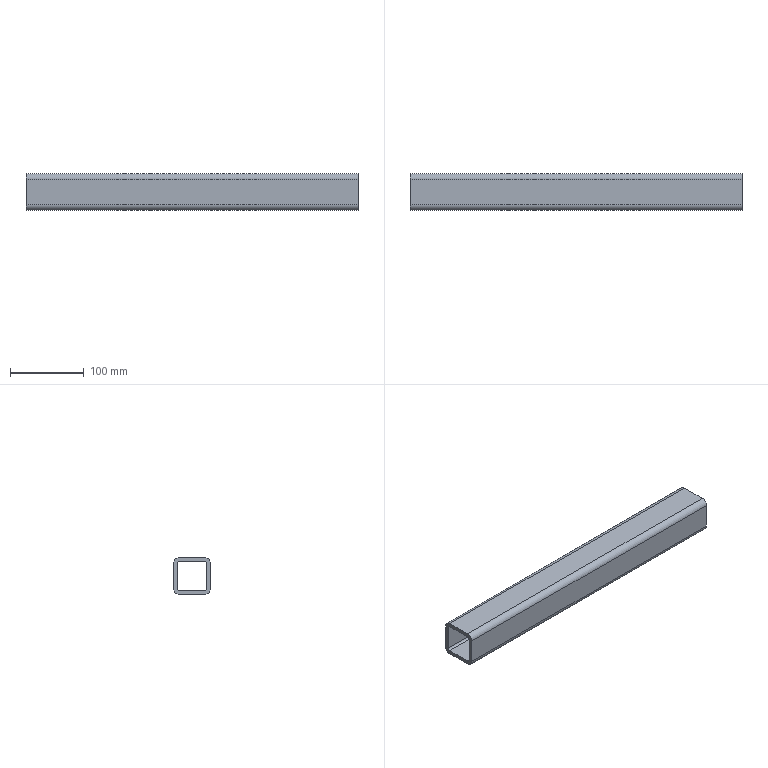Part | SolidWorks | features WeldMemberFeat 1, WeldmentFeature 1 | 1 solid | 18 faces | box 450 x 50 x 50 mm | volume 383754 mm3 | plane 10 | cylinder 8 | commonest cylinder face diameters 6 x4 16 x4
STEP:
#1=CARTESIAN_POINT('',(-88.434,25.,17.));
#2=VERTEX_POINT('',#1);
#3=CARTESIAN_POINT('',(-88.434,17.,25.));
#4=VERTEX_POINT('',#3);
#5=CARTESIAN_POINT('',(-88.434,17.,17.));
#6=DIRECTION('',(1.,0.,0.));
#7=DIRECTION('',(0.,0.,-1.));
#8=AXIS2_PLACEMENT_3D('',#5,#6,#7);
#9=CIRCLE('',#8,8.);
#10=EDGE_CURVE('',#2,#4,#9,.T.);
#11=ORIENTED_EDGE('',*,*,#10,.T.);
#12=CARTESIAN_POINT('',(361.566,17.,25.));
#13=VERTEX_POINT('',#12);
#14=CARTESIAN_POINT('',(361.566,17.,25.));
#15=DIRECTION('',(-1.,0.,0.));
#16=VECTOR('',#15,1000.);
#17=LINE('',#14,#16);
#18=EDGE_CURVE('',#13,#4,#17,.T.);
#19=ORIENTED_EDGE('',*,*,#18,.F.);
#20=CARTESIAN_POINT('',(361.566,25.,17.));
#21=VERTEX_POINT('',#20);
#22=CARTESIAN_POINT('',(361.566,17.,17.));
#23=DIRECTION('',(1.,0.,0.));
#24=DIRECTION('',(0.,0.,-1.));
#25=AXIS2_PLACEMENT_3D('',#22,#23,#24);
#26=CIRCLE('',#25,8.);
#27=EDGE_CURVE('',#21,#13,#26,.T.);
#28=ORIENTED_EDGE('',*,*,#27,.F.);
#29=CARTESIAN_POINT('',(361.566,25.,17.));
#30=DIRECTION('',(-1.,0.,0.));
#31=VECTOR('',#30,1000.);
#32=LINE('',#29,#31);
#33=EDGE_CURVE('',#21,#2,#32,.T.);
#34=ORIENTED_EDGE('',*,*,#33,.T.);
#35=EDGE_LOOP('',(#11,#19,#28,#34));
#36=FACE_OUTER_BOUND('',#35,.T.);
#37=CARTESIAN_POINT('',(361.566,17.,17.));
#38=DIRECTION('',(-1.,0.,0.));
#39=DIRECTION('',(0.,0.,1.));
#40=AXIS2_PLACEMENT_3D('',#37,#38,#39);
#41=CYLINDRICAL_SURFACE('',#40,8.);
#42=ADVANCED_FACE('',(#36),#41,.T.);
#43=CARTESIAN_POINT('',(-88.434,-17.,25.));
#44=VERTEX_POINT('',#43);
#45=CARTESIAN_POINT('',(-88.434,17.,25.));
#46=DIRECTION('',(0.,-1.,0.));
#47=VECTOR('',#46,1000.);
#48=LINE('',#45,#47);
#49=EDGE_CURVE('',#4,#44,#48,.T.);
#50=ORIENTED_EDGE('',*,*,#49,.T.);
#51=CARTESIAN_POINT('',(361.566,-17.,25.));
#52=VERTEX_POINT('',#51);
#53=CARTESIAN_POINT('',(361.566,-17.,25.));
#54=DIRECTION('',(-1.,0.,0.));
#55=VECTOR('',#54,1000.);
#56=LINE('',#53,#55);
#57=EDGE_CURVE('',#52,#44,#56,.T.);
#58=ORIENTED_EDGE('',*,*,#57,.F.);
#59=CARTESIAN_POINT('',(361.566,17.,25.));
#60=DIRECTION('',(0.,-1.,0.));
#61=VECTOR('',#60,1000.);
#62=LINE('',#59,#61);
#63=EDGE_CURVE('',#13,#52,#62,.T.);
#64=ORIENTED_EDGE('',*,*,#63,.F.);
#65=ORIENTED_EDGE('',*,*,#18,.T.);
#66=EDGE_LOOP('',(#50,#58,#64,#65));
#67=FACE_OUTER_BOUND('',#66,.T.);
#68=CARTESIAN_POINT('',(361.566,17.,25.));
#69=DIRECTION('',(0.,0.,-1.));
#70=DIRECTION('',(-1.,0.,0.));
#71=AXIS2_PLACEMENT_3D('',#68,#69,#70);
#72=PLANE('',#71);
#73=ADVANCED_FACE('',(#67),#72,.F.);
#74=CARTESIAN_POINT('',(-88.434,-25.,17.));
#75=VERTEX_POINT('',#74);
#76=CARTESIAN_POINT('',(-88.434,-17.,17.));
#77=DIRECTION('',(1.,0.,0.));
#78=DIRECTION('',(0.,0.,-1.));
#79=AXIS2_PLACEMENT_3D('',#76,#77,#78);
#80=CIRCLE('',#79,8.);
#81=EDGE_CURVE('',#44,#75,#80,.T.);
#82=ORIENTED_EDGE('',*,*,#81,.T.);
#83=CARTESIAN_POINT('',(361.566,-25.,17.));
#84=VERTEX_POINT('',#83);
#85=CARTESIAN_POINT('',(361.566,-25.,17.));
#86=DIRECTION('',(-1.,0.,0.));
#87=VECTOR('',#86,1000.);
#88=LINE('',#85,#87);
#89=EDGE_CURVE('',#84,#75,#88,.T.);
#90=ORIENTED_EDGE('',*,*,#89,.F.);
#91=CARTESIAN_POINT('',(361.566,-17.,17.));
#92=DIRECTION('',(1.,0.,0.));
#93=DIRECTION('',(0.,0.,-1.));
#94=AXIS2_PLACEMENT_3D('',#91,#92,#93);
#95=CIRCLE('',#94,8.);
#96=EDGE_CURVE('',#52,#84,#95,.T.);
#97=ORIENTED_EDGE('',*,*,#96,.F.);
#98=ORIENTED_EDGE('',*,*,#57,.T.);
#99=EDGE_LOOP('',(#82,#90,#97,#98));
#100=FACE_OUTER_BOUND('',#99,.T.);
#101=CARTESIAN_POINT('',(361.566,-17.,17.));
#102=DIRECTION('',(-1.,0.,0.));
#103=DIRECTION('',(0.,0.,1.));
#104=AXIS2_PLACEMENT_3D('',#101,#102,#103);
#105=CYLINDRICAL_SURFACE('',#104,8.);
#106=ADVANCED_FACE('',(#100),#105,.T.);
#107=CARTESIAN_POINT('',(-88.434,-25.,-17.));
#108=VERTEX_POINT('',#107);
#109=CARTESIAN_POINT('',(-88.434,-25.,-17.));
#110=DIRECTION('',(0.,0.,-1.));
#111=VECTOR('',#110,1000.);
#112=LINE('',#109,#111);
#113=EDGE_CURVE('',#75,#108,#112,.T.);
#114=ORIENTED_EDGE('',*,*,#113,.T.);
#115=CARTESIAN_POINT('',(361.566,-25.,-17.));
#116=VERTEX_POINT('',#115);
#117=CARTESIAN_POINT('',(361.566,-25.,-17.));
#118=DIRECTION('',(-1.,0.,0.));
#119=VECTOR('',#118,1000.);
#120=LINE('',#117,#119);
#121=EDGE_CURVE('',#116,#108,#120,.T.);
#122=ORIENTED_EDGE('',*,*,#121,.F.);
#123=CARTESIAN_POINT('',(361.566,-25.,-17.));
#124=DIRECTION('',(0.,0.,-1.));
#125=VECTOR('',#124,1000.);
#126=LINE('',#123,#125);
#127=EDGE_CURVE('',#84,#116,#126,.T.);
#128=ORIENTED_EDGE('',*,*,#127,.F.);
#129=ORIENTED_EDGE('',*,*,#89,.T.);
#130=EDGE_LOOP('',(#114,#122,#128,#129));
#131=FACE_OUTER_BOUND('',#130,.T.);
#132=CARTESIAN_POINT('',(361.566,-25.,-17.));
#133=DIRECTION('',(0.,1.,0.));
#134=DIRECTION('',(0.,0.,1.));
#135=AXIS2_PLACEMENT_3D('',#132,#133,#134);
#136=PLANE('',#135);
#137=ADVANCED_FACE('',(#131),#136,.F.);
#138=CARTESIAN_POINT('',(-88.434,-17.,-25.));
#139=VERTEX_POINT('',#138);
#140=CARTESIAN_POINT('',(-88.434,-17.,-17.));
#141=DIRECTION('',(1.,0.,0.));
#142=DIRECTION('',(0.,0.,-1.));
#143=AXIS2_PLACEMENT_3D('',#140,#141,#142);
#144=CIRCLE('',#143,8.);
#145=EDGE_CURVE('',#108,#139,#144,.T.);
#146=ORIENTED_EDGE('',*,*,#145,.T.);
#147=CARTESIAN_POINT('',(361.566,-17.,-25.));
#148=VERTEX_POINT('',#147);
#149=CARTESIAN_POINT('',(361.566,-17.,-25.));
#150=DIRECTION('',(-1.,0.,0.));
#151=VECTOR('',#150,1000.);
#152=LINE('',#149,#151);
#153=EDGE_CURVE('',#148,#139,#152,.T.);
#154=ORIENTED_EDGE('',*,*,#153,.F.);
#155=CARTESIAN_POINT('',(361.566,-17.,-17.));
#156=DIRECTION('',(1.,0.,0.));
#157=DIRECTION('',(0.,0.,-1.));
#158=AXIS2_PLACEMENT_3D('',#155,#156,#157);
#159=CIRCLE('',#158,8.);
#160=EDGE_CURVE('',#116,#148,#159,.T.);
#161=ORIENTED_EDGE('',*,*,#160,.F.);
#162=ORIENTED_EDGE('',*,*,#121,.T.);
#163=EDGE_LOOP('',(#146,#154,#161,#162));
#164=FACE_OUTER_BOUND('',#163,.T.);
#165=CARTESIAN_POINT('',(361.566,-17.,-17.));
#166=DIRECTION('',(-1.,0.,0.));
#167=DIRECTION('',(0.,0.,1.));
#168=AXIS2_PLACEMENT_3D('',#165,#166,#167);
#169=CYLINDRICAL_SURFACE('',#168,8.);
#170=ADVANCED_FACE('',(#164),#169,.T.);
#171=CARTESIAN_POINT('',(-88.434,17.,-25.));
#172=VERTEX_POINT('',#171);
#173=CARTESIAN_POINT('',(-88.434,-17.,-25.));
#174=DIRECTION('',(0.,1.,0.));
#175=VECTOR('',#174,1000.);
#176=LINE('',#173,#175);
#177=EDGE_CURVE('',#139,#172,#176,.T.);
#178=ORIENTED_EDGE('',*,*,#177,.T.);
#179=CARTESIAN_POINT('',(361.566,17.,-25.));
#180=VERTEX_POINT('',#179);
#181=CARTESIAN_POINT('',(361.566,17.,-25.));
#182=DIRECTION('',(-1.,0.,0.));
#183=VECTOR('',#182,1000.);
#184=LINE('',#181,#183);
#185=EDGE_CURVE('',#180,#172,#184,.T.);
#186=ORIENTED_EDGE('',*,*,#185,.F.);
#187=CARTESIAN_POINT('',(361.566,-17.,-25.));
#188=DIRECTION('',(0.,1.,0.));
#189=VECTOR('',#188,1000.);
#190=LINE('',#187,#189);
#191=EDGE_CURVE('',#148,#180,#190,.T.);
#192=ORIENTED_EDGE('',*,*,#191,.F.);
#193=ORIENTED_EDGE('',*,*,#153,.T.);
#194=EDGE_LOOP('',(#178,#186,#192,#193));
#195=FACE_OUTER_BOUND('',#194,.T.);
#196=CARTESIAN_POINT('',(361.566,-17.,-25.));
#197=DIRECTION('',(0.,0.,1.));
#198=DIRECTION('',(1.,0.,0.));
#199=AXIS2_PLACEMENT_3D('',#196,#197,#198);
#200=PLANE('',#199);
#201=ADVANCED_FACE('',(#195),#200,.F.);
#202=CARTESIAN_POINT('',(-88.434,25.,-17.));
#203=VERTEX_POINT('',#202);
#204=CARTESIAN_POINT('',(-88.434,17.,-17.));
#205=DIRECTION('',(1.,0.,0.));
#206=DIRECTION('',(0.,0.,-1.));
#207=AXIS2_PLACEMENT_3D('',#204,#205,#206);
#208=CIRCLE('',#207,8.);
#209=EDGE_CURVE('',#172,#203,#208,.T.);
#210=ORIENTED_EDGE('',*,*,#209,.T.);
#211=CARTESIAN_POINT('',(361.566,25.,-17.));
#212=VERTEX_POINT('',#211);
#213=CARTESIAN_POINT('',(361.566,25.,-17.));
#214=DIRECTION('',(-1.,0.,0.));
#215=VECTOR('',#214,1000.);
#216=LINE('',#213,#215);
#217=EDGE_CURVE('',#212,#203,#216,.T.);
#218=ORIENTED_EDGE('',*,*,#217,.F.);
#219=CARTESIAN_POINT('',(361.566,17.,-17.));
#220=DIRECTION('',(1.,0.,0.));
#221=DIRECTION('',(0.,0.,-1.));
#222=AXIS2_PLACEMENT_3D('',#219,#220,#221);
#223=CIRCLE('',#222,8.);
#224=EDGE_CURVE('',#180,#212,#223,.T.);
#225=ORIENTED_EDGE('',*,*,#224,.F.);
#226=ORIENTED_EDGE('',*,*,#185,.T.);
#227=EDGE_LOOP('',(#210,#218,#225,#226));
#228=FACE_OUTER_BOUND('',#227,.T.);
#229=CARTESIAN_POINT('',(361.566,17.,-17.));
#230=DIRECTION('',(-1.,0.,0.));
#231=DIRECTION('',(0.,0.,1.));
#232=AXIS2_PLACEMENT_3D('',#229,#230,#231);
#233=CYLINDRICAL_SURFACE('',#232,8.);
#234=ADVANCED_FACE('',(#228),#233,.T.);
#235=CARTESIAN_POINT('',(-88.434,-17.,20.));
#236=VERTEX_POINT('',#235);
#237=CARTESIAN_POINT('',(-88.434,-20.,17.));
#238=VERTEX_POINT('',#237);
#239=CARTESIAN_POINT('',(-88.434,-17.,17.));
#240=DIRECTION('',(1.,0.,0.));
#241=DIRECTION('',(0.,0.,-1.));
#242=AXIS2_PLACEMENT_3D('',#239,#240,#241);
#243=CIRCLE('',#242,3.);
#244=EDGE_CURVE('',#236,#238,#243,.T.);
#245=ORIENTED_EDGE('',*,*,#244,.F.);
#246=CARTESIAN_POINT('',(361.566,-17.,20.));
#247=VERTEX_POINT('',#246);
#248=CARTESIAN_POINT('',(361.566,-17.,20.));
#249=DIRECTION('',(-1.,0.,0.));
#250=VECTOR('',#249,1000.);
#251=LINE('',#248,#250);
#252=EDGE_CURVE('',#247,#236,#251,.T.);
#253=ORIENTED_EDGE('',*,*,#252,.F.);
#254=CARTESIAN_POINT('',(361.566,-20.,17.));
#255=VERTEX_POINT('',#254);
#256=CARTESIAN_POINT('',(361.566,-17.,17.));
#257=DIRECTION('',(1.,0.,0.));
#258=DIRECTION('',(0.,0.,-1.));
#259=AXIS2_PLACEMENT_3D('',#256,#257,#258);
#260=CIRCLE('',#259,3.);
#261=EDGE_CURVE('',#247,#255,#260,.T.);
#262=ORIENTED_EDGE('',*,*,#261,.T.);
#263=CARTESIAN_POINT('',(361.566,-20.,17.));
#264=DIRECTION('',(-1.,0.,0.));
#265=VECTOR('',#264,1000.);
#266=LINE('',#263,#265);
#267=EDGE_CURVE('',#255,#238,#266,.T.);
#268=ORIENTED_EDGE('',*,*,#267,.T.);
#269=EDGE_LOOP('',(#245,#253,#262,#268));
#270=FACE_OUTER_BOUND('',#269,.T.);
#271=CARTESIAN_POINT('',(361.566,-17.,17.));
#272=DIRECTION('',(-1.,0.,0.));
#273=DIRECTION('',(0.,0.,1.));
#274=AXIS2_PLACEMENT_3D('',#271,#272,#273);
#275=CYLINDRICAL_SURFACE('',#274,3.);
#276=ADVANCED_FACE('',(#270),#275,.F.);
#277=CARTESIAN_POINT('',(-88.434,17.,20.));
#278=VERTEX_POINT('',#277);
#279=CARTESIAN_POINT('',(-88.434,17.,20.));
#280=DIRECTION('',(0.,-1.,0.));
#281=VECTOR('',#280,1000.);
#282=LINE('',#279,#281);
#283=EDGE_CURVE('',#278,#236,#282,.T.);
#284=ORIENTED_EDGE('',*,*,#283,.F.);
#285=CARTESIAN_POINT('',(361.566,17.,20.));
#286=VERTEX_POINT('',#285);
#287=CARTESIAN_POINT('',(361.566,17.,20.));
#288=DIRECTION('',(-1.,0.,0.));
#289=VECTOR('',#288,1000.);
#290=LINE('',#287,#289);
#291=EDGE_CURVE('',#286,#278,#290,.T.);
#292=ORIENTED_EDGE('',*,*,#291,.F.);
#293=CARTESIAN_POINT('',(361.566,17.,20.));
#294=DIRECTION('',(0.,-1.,0.));
#295=VECTOR('',#294,1000.);
#296=LINE('',#293,#295);
#297=EDGE_CURVE('',#286,#247,#296,.T.);
#298=ORIENTED_EDGE('',*,*,#297,.T.);
#299=ORIENTED_EDGE('',*,*,#252,.T.);
#300=EDGE_LOOP('',(#284,#292,#298,#299));
#301=FACE_OUTER_BOUND('',#300,.T.);
#302=CARTESIAN_POINT('',(361.566,17.,20.));
#303=DIRECTION('',(0.,0.,-1.));
#304=DIRECTION('',(-1.,0.,0.));
#305=AXIS2_PLACEMENT_3D('',#302,#303,#304);
#306=PLANE('',#305);
#307=ADVANCED_FACE('',(#301),#306,.T.);
#308=CARTESIAN_POINT('',(-88.434,20.,17.));
#309=VERTEX_POINT('',#308);
#310=CARTESIAN_POINT('',(-88.434,17.,17.));
#311=DIRECTION('',(1.,0.,0.));
#312=DIRECTION('',(0.,0.,-1.));
#313=AXIS2_PLACEMENT_3D('',#310,#311,#312);
#314=CIRCLE('',#313,3.);
#315=EDGE_CURVE('',#309,#278,#314,.T.);
#316=ORIENTED_EDGE('',*,*,#315,.F.);
#317=CARTESIAN_POINT('',(361.566,20.,17.));
#318=VERTEX_POINT('',#317);
#319=CARTESIAN_POINT('',(361.566,20.,17.));
#320=DIRECTION('',(-1.,0.,0.));
#321=VECTOR('',#320,1000.);
#322=LINE('',#319,#321);
#323=EDGE_CURVE('',#318,#309,#322,.T.);
#324=ORIENTED_EDGE('',*,*,#323,.F.);
#325=CARTESIAN_POINT('',(361.566,17.,17.));
#326=DIRECTION('',(1.,0.,0.));
#327=DIRECTION('',(0.,0.,-1.));
#328=AXIS2_PLACEMENT_3D('',#325,#326,#327);
#329=CIRCLE('',#328,3.);
#330=EDGE_CURVE('',#318,#286,#329,.T.);
#331=ORIENTED_EDGE('',*,*,#330,.T.);
#332=ORIENTED_EDGE('',*,*,#291,.T.);
#333=EDGE_LOOP('',(#316,#324,#331,#332));
#334=FACE_OUTER_BOUND('',#333,.T.);
#335=CARTESIAN_POINT('',(361.566,17.,17.));
#336=DIRECTION('',(-1.,0.,0.));
#337=DIRECTION('',(0.,0.,1.));
#338=AXIS2_PLACEMENT_3D('',#335,#336,#337);
#339=CYLINDRICAL_SURFACE('',#338,3.);
#340=ADVANCED_FACE('',(#334),#339,.F.);
#341=CARTESIAN_POINT('',(-88.434,20.,-17.));
#342=VERTEX_POINT('',#341);
#343=CARTESIAN_POINT('',(-88.434,20.,17.));
#344=DIRECTION('',(0.,0.,1.));
#345=VECTOR('',#344,1000.);
#346=LINE('',#343,#345);
#347=EDGE_CURVE('',#342,#309,#346,.T.);
#348=ORIENTED_EDGE('',*,*,#347,.F.);
#349=CARTESIAN_POINT('',(361.566,20.,-17.));
#350=VERTEX_POINT('',#349);
#351=CARTESIAN_POINT('',(361.566,20.,-17.));
#352=DIRECTION('',(-1.,0.,0.));
#353=VECTOR('',#352,1000.);
#354=LINE('',#351,#353);
#355=EDGE_CURVE('',#350,#342,#354,.T.);
#356=ORIENTED_EDGE('',*,*,#355,.F.);
#357=CARTESIAN_POINT('',(361.566,20.,17.));
#358=DIRECTION('',(0.,0.,1.));
#359=VECTOR('',#358,1000.);
#360=LINE('',#357,#359);
#361=EDGE_CURVE('',#350,#318,#360,.T.);
#362=ORIENTED_EDGE('',*,*,#361,.T.);
#363=ORIENTED_EDGE('',*,*,#323,.T.);
#364=EDGE_LOOP('',(#348,#356,#362,#363));
#365=FACE_OUTER_BOUND('',#364,.T.);
#366=CARTESIAN_POINT('',(361.566,20.,17.));
#367=DIRECTION('',(0.,-1.,0.));
#368=DIRECTION('',(0.,0.,-1.));
#369=AXIS2_PLACEMENT_3D('',#366,#367,#368);
#370=PLANE('',#369);
#371=ADVANCED_FACE('',(#365),#370,.T.);
#372=CARTESIAN_POINT('',(-88.434,17.,-20.));
#373=VERTEX_POINT('',#372);
#374=CARTESIAN_POINT('',(-88.434,17.,-17.));
#375=DIRECTION('',(1.,0.,0.));
#376=DIRECTION('',(0.,0.,-1.));
#377=AXIS2_PLACEMENT_3D('',#374,#375,#376);
#378=CIRCLE('',#377,3.);
#379=EDGE_CURVE('',#373,#342,#378,.T.);
#380=ORIENTED_EDGE('',*,*,#379,.F.);
#381=CARTESIAN_POINT('',(361.566,17.,-20.));
#382=VERTEX_POINT('',#381);
#383=CARTESIAN_POINT('',(361.566,17.,-20.));
#384=DIRECTION('',(-1.,0.,0.));
#385=VECTOR('',#384,1000.);
#386=LINE('',#383,#385);
#387=EDGE_CURVE('',#382,#373,#386,.T.);
#388=ORIENTED_EDGE('',*,*,#387,.F.);
#389=CARTESIAN_POINT('',(361.566,17.,-17.));
#390=DIRECTION('',(1.,0.,0.));
#391=DIRECTION('',(0.,0.,-1.));
#392=AXIS2_PLACEMENT_3D('',#389,#390,#391);
#393=CIRCLE('',#392,3.);
#394=EDGE_CURVE('',#382,#350,#393,.T.);
#395=ORIENTED_EDGE('',*,*,#394,.T.);
#396=ORIENTED_EDGE('',*,*,#355,.T.);
#397=EDGE_LOOP('',(#380,#388,#395,#396));
#398=FACE_OUTER_BOUND('',#397,.T.);
#399=CARTESIAN_POINT('',(361.566,17.,-17.));
#400=DIRECTION('',(-1.,0.,0.));
#401=DIRECTION('',(0.,0.,1.));
#402=AXIS2_PLACEMENT_3D('',#399,#400,#401);
#403=CYLINDRICAL_SURFACE('',#402,3.);
#404=ADVANCED_FACE('',(#398),#403,.F.);
#405=CARTESIAN_POINT('',(-88.434,-17.,-20.));
#406=VERTEX_POINT('',#405);
#407=CARTESIAN_POINT('',(-88.434,-17.,-20.));
#408=DIRECTION('',(0.,1.,0.));
#409=VECTOR('',#408,1000.);
#410=LINE('',#407,#409);
#411=EDGE_CURVE('',#406,#373,#410,.T.);
#412=ORIENTED_EDGE('',*,*,#411,.F.);
#413=CARTESIAN_POINT('',(361.566,-17.,-20.));
#414=VERTEX_POINT('',#413);
#415=CARTESIAN_POINT('',(361.566,-17.,-20.));
#416=DIRECTION('',(-1.,0.,0.));
#417=VECTOR('',#416,1000.);
#418=LINE('',#415,#417);
#419=EDGE_CURVE('',#414,#406,#418,.T.);
#420=ORIENTED_EDGE('',*,*,#419,.F.);
#421=CARTESIAN_POINT('',(361.566,-17.,-20.));
#422=DIRECTION('',(0.,1.,0.));
#423=VECTOR('',#422,1000.);
#424=LINE('',#421,#423);
#425=EDGE_CURVE('',#414,#382,#424,.T.);
#426=ORIENTED_EDGE('',*,*,#425,.T.);
#427=ORIENTED_EDGE('',*,*,#387,.T.);
#428=EDGE_LOOP('',(#412,#420,#426,#427));
#429=FACE_OUTER_BOUND('',#428,.T.);
#430=CARTESIAN_POINT('',(361.566,-17.,-20.));
#431=DIRECTION('',(0.,0.,1.));
#432=DIRECTION('',(1.,0.,0.));
#433=AXIS2_PLACEMENT_3D('',#430,#431,#432);
#434=PLANE('',#433);
#435=ADVANCED_FACE('',(#429),#434,.T.);
#436=CARTESIAN_POINT('',(-88.434,-20.,-17.));
#437=VERTEX_POINT('',#436);
#438=CARTESIAN_POINT('',(-88.434,-17.,-17.));
#439=DIRECTION('',(1.,0.,0.));
#440=DIRECTION('',(0.,0.,-1.));
#441=AXIS2_PLACEMENT_3D('',#438,#439,#440);
#442=CIRCLE('',#441,3.);
#443=EDGE_CURVE('',#437,#406,#442,.T.);
#444=ORIENTED_EDGE('',*,*,#443,.F.);
#445=CARTESIAN_POINT('',(361.566,-20.,-17.));
#446=VERTEX_POINT('',#445);
#447=CARTESIAN_POINT('',(361.566,-20.,-17.));
#448=DIRECTION('',(-1.,0.,0.));
#449=VECTOR('',#448,1000.);
#450=LINE('',#447,#449);
#451=EDGE_CURVE('',#446,#437,#450,.T.);
#452=ORIENTED_EDGE('',*,*,#451,.F.);
#453=CARTESIAN_POINT('',(361.566,-17.,-17.));
#454=DIRECTION('',(1.,0.,0.));
#455=DIRECTION('',(0.,0.,-1.));
#456=AXIS2_PLACEMENT_3D('',#453,#454,#455);
#457=CIRCLE('',#456,3.);
#458=EDGE_CURVE('',#446,#414,#457,.T.);
#459=ORIENTED_EDGE('',*,*,#458,.T.);
#460=ORIENTED_EDGE('',*,*,#419,.T.);
#461=EDGE_LOOP('',(#444,#452,#459,#460));
#462=FACE_OUTER_BOUND('',#461,.T.);
#463=CARTESIAN_POINT('',(361.566,-17.,-17.));
#464=DIRECTION('',(-1.,0.,0.));
#465=DIRECTION('',(0.,0.,1.));
#466=AXIS2_PLACEMENT_3D('',#463,#464,#465);
#467=CYLINDRICAL_SURFACE('',#466,3.);
#468=ADVANCED_FACE('',(#462),#467,.F.);
#469=CARTESIAN_POINT('',(-88.434,-20.,-17.));
#470=DIRECTION('',(0.,0.,-1.));
#471=VECTOR('',#470,1000.);
#472=LINE('',#469,#471);
#473=EDGE_CURVE('',#238,#437,#472,.T.);
#474=ORIENTED_EDGE('',*,*,#473,.F.);
#475=ORIENTED_EDGE('',*,*,#267,.F.);
#476=CARTESIAN_POINT('',(361.566,-20.,-17.));
#477=DIRECTION('',(0.,0.,-1.));
#478=VECTOR('',#477,1000.);
#479=LINE('',#476,#478);
#480=EDGE_CURVE('',#255,#446,#479,.T.);
#481=ORIENTED_EDGE('',*,*,#480,.T.);
#482=ORIENTED_EDGE('',*,*,#451,.T.);
#483=EDGE_LOOP('',(#474,#475,#481,#482));
#484=FACE_OUTER_BOUND('',#483,.T.);
#485=CARTESIAN_POINT('',(361.566,-20.,-17.));
#486=DIRECTION('',(0.,1.,0.));
#487=DIRECTION('',(0.,0.,1.));
#488=AXIS2_PLACEMENT_3D('',#485,#486,#487);
#489=PLANE('',#488);
#490=ADVANCED_FACE('',(#484),#489,.T.);
#491=CARTESIAN_POINT('',(-88.434,25.,17.));
#492=DIRECTION('',(0.,0.,1.));
#493=VECTOR('',#492,1000.);
#494=LINE('',#491,#493);
#495=EDGE_CURVE('',#203,#2,#494,.T.);
#496=ORIENTED_EDGE('',*,*,#495,.T.);
#497=ORIENTED_EDGE('',*,*,#33,.F.);
#498=CARTESIAN_POINT('',(361.566,25.,17.));
#499=DIRECTION('',(0.,0.,1.));
#500=VECTOR('',#499,1000.);
#501=LINE('',#498,#500);
#502=EDGE_CURVE('',#212,#21,#501,.T.);
#503=ORIENTED_EDGE('',*,*,#502,.F.);
#504=ORIENTED_EDGE('',*,*,#217,.T.);
#505=EDGE_LOOP('',(#496,#497,#503,#504));
#506=FACE_OUTER_BOUND('',#505,.T.);
#507=CARTESIAN_POINT('',(361.566,25.,17.));
#508=DIRECTION('',(0.,-1.,0.));
#509=DIRECTION('',(0.,0.,-1.));
#510=AXIS2_PLACEMENT_3D('',#507,#508,#509);
#511=PLANE('',#510);
#512=ADVANCED_FACE('',(#506),#511,.F.);
#513=ORIENTED_EDGE('',*,*,#261,.F.);
#514=ORIENTED_EDGE('',*,*,#297,.F.);
#515=ORIENTED_EDGE('',*,*,#330,.F.);
#516=ORIENTED_EDGE('',*,*,#361,.F.);
#517=ORIENTED_EDGE('',*,*,#394,.F.);
#518=ORIENTED_EDGE('',*,*,#425,.F.);
#519=ORIENTED_EDGE('',*,*,#458,.F.);
#520=ORIENTED_EDGE('',*,*,#480,.F.);
#521=EDGE_LOOP('',(#513,#514,#515,#516,#517,#518,#519,#520));
#522=FACE_BOUND('',#521,.T.);
#523=ORIENTED_EDGE('',*,*,#27,.T.);
#524=ORIENTED_EDGE('',*,*,#63,.T.);
#525=ORIENTED_EDGE('',*,*,#96,.T.);
#526=ORIENTED_EDGE('',*,*,#127,.T.);
#527=ORIENTED_EDGE('',*,*,#160,.T.);
#528=ORIENTED_EDGE('',*,*,#191,.T.);
#529=ORIENTED_EDGE('',*,*,#224,.T.);
#530=ORIENTED_EDGE('',*,*,#502,.T.);
#531=EDGE_LOOP('',(#523,#524,#525,#526,#527,#528,#529,#530));
#532=FACE_OUTER_BOUND('',#531,.T.);
#533=CARTESIAN_POINT('',(361.566,17.,17.));
#534=DIRECTION('',(1.,0.,0.));
#535=DIRECTION('',(0.,0.,-1.));
#536=AXIS2_PLACEMENT_3D('',#533,#534,#535);
#537=PLANE('',#536);
#538=ADVANCED_FACE('',(#522,#532),#537,.T.);
#539=ORIENTED_EDGE('',*,*,#244,.T.);
#540=ORIENTED_EDGE('',*,*,#473,.T.);
#541=ORIENTED_EDGE('',*,*,#443,.T.);
#542=ORIENTED_EDGE('',*,*,#411,.T.);
#543=ORIENTED_EDGE('',*,*,#379,.T.);
#544=ORIENTED_EDGE('',*,*,#347,.T.);
#545=ORIENTED_EDGE('',*,*,#315,.T.);
#546=ORIENTED_EDGE('',*,*,#283,.T.);
#547=EDGE_LOOP('',(#539,#540,#541,#542,#543,#544,#545,#546));
#548=FACE_BOUND('',#547,.T.);
#549=ORIENTED_EDGE('',*,*,#10,.F.);
#550=ORIENTED_EDGE('',*,*,#495,.F.);
#551=ORIENTED_EDGE('',*,*,#209,.F.);
#552=ORIENTED_EDGE('',*,*,#177,.F.);
#553=ORIENTED_EDGE('',*,*,#145,.F.);
#554=ORIENTED_EDGE('',*,*,#113,.F.);
#555=ORIENTED_EDGE('',*,*,#81,.F.);
#556=ORIENTED_EDGE('',*,*,#49,.F.);
#557=EDGE_LOOP('',(#549,#550,#551,#552,#553,#554,#555,#556));
#558=FACE_OUTER_BOUND('',#557,.T.);
#559=CARTESIAN_POINT('',(-88.434,17.,17.));
#560=DIRECTION('',(1.,0.,0.));
#561=DIRECTION('',(0.,0.,-1.));
#562=AXIS2_PLACEMENT_3D('',#559,#560,#561);
#563=PLANE('',#562);
#564=ADVANCED_FACE('',(#548,#558),#563,.F.);
#565=CLOSED_SHELL('',(#42,#73,#106,#137,#170,#201,#234,#276,#307,#340,#371,#404,#435,#468,#490,#512,#538,#564));
#566=MANIFOLD_SOLID_BREP('',#565);
#567=CARTESIAN_POINT('',(0.,0.,0.));
#568=DIRECTION('',(0.,0.,1.));
#569=DIRECTION('',(1.,0.,0.));
#570=AXIS2_PLACEMENT_3D('',#567,#568,#569);
#571=(LENGTH_UNIT()NAMED_UNIT(*)SI_UNIT(.MILLI.,.METRE.));
#572=UNCERTAINTY_MEASURE_WITH_UNIT(LENGTH_MEASURE(0.00001),#571,'','');
#573=(NAMED_UNIT(*)PLANE_ANGLE_UNIT()SI_UNIT($,.RADIAN.));
#574=(NAMED_UNIT(*)SI_UNIT($,.STERADIAN.)SOLID_ANGLE_UNIT());
#575=(GEOMETRIC_REPRESENTATION_CONTEXT(3)GLOBAL_UNCERTAINTY_ASSIGNED_CONTEXT((#572))GLOBAL_UNIT_ASSIGNED_CONTEXT((#571,#573,#574))REPRESENTATION_CONTEXT('',''));
#576=ADVANCED_BREP_SHAPE_REPRESENTATION('',(#566,#570),#575);